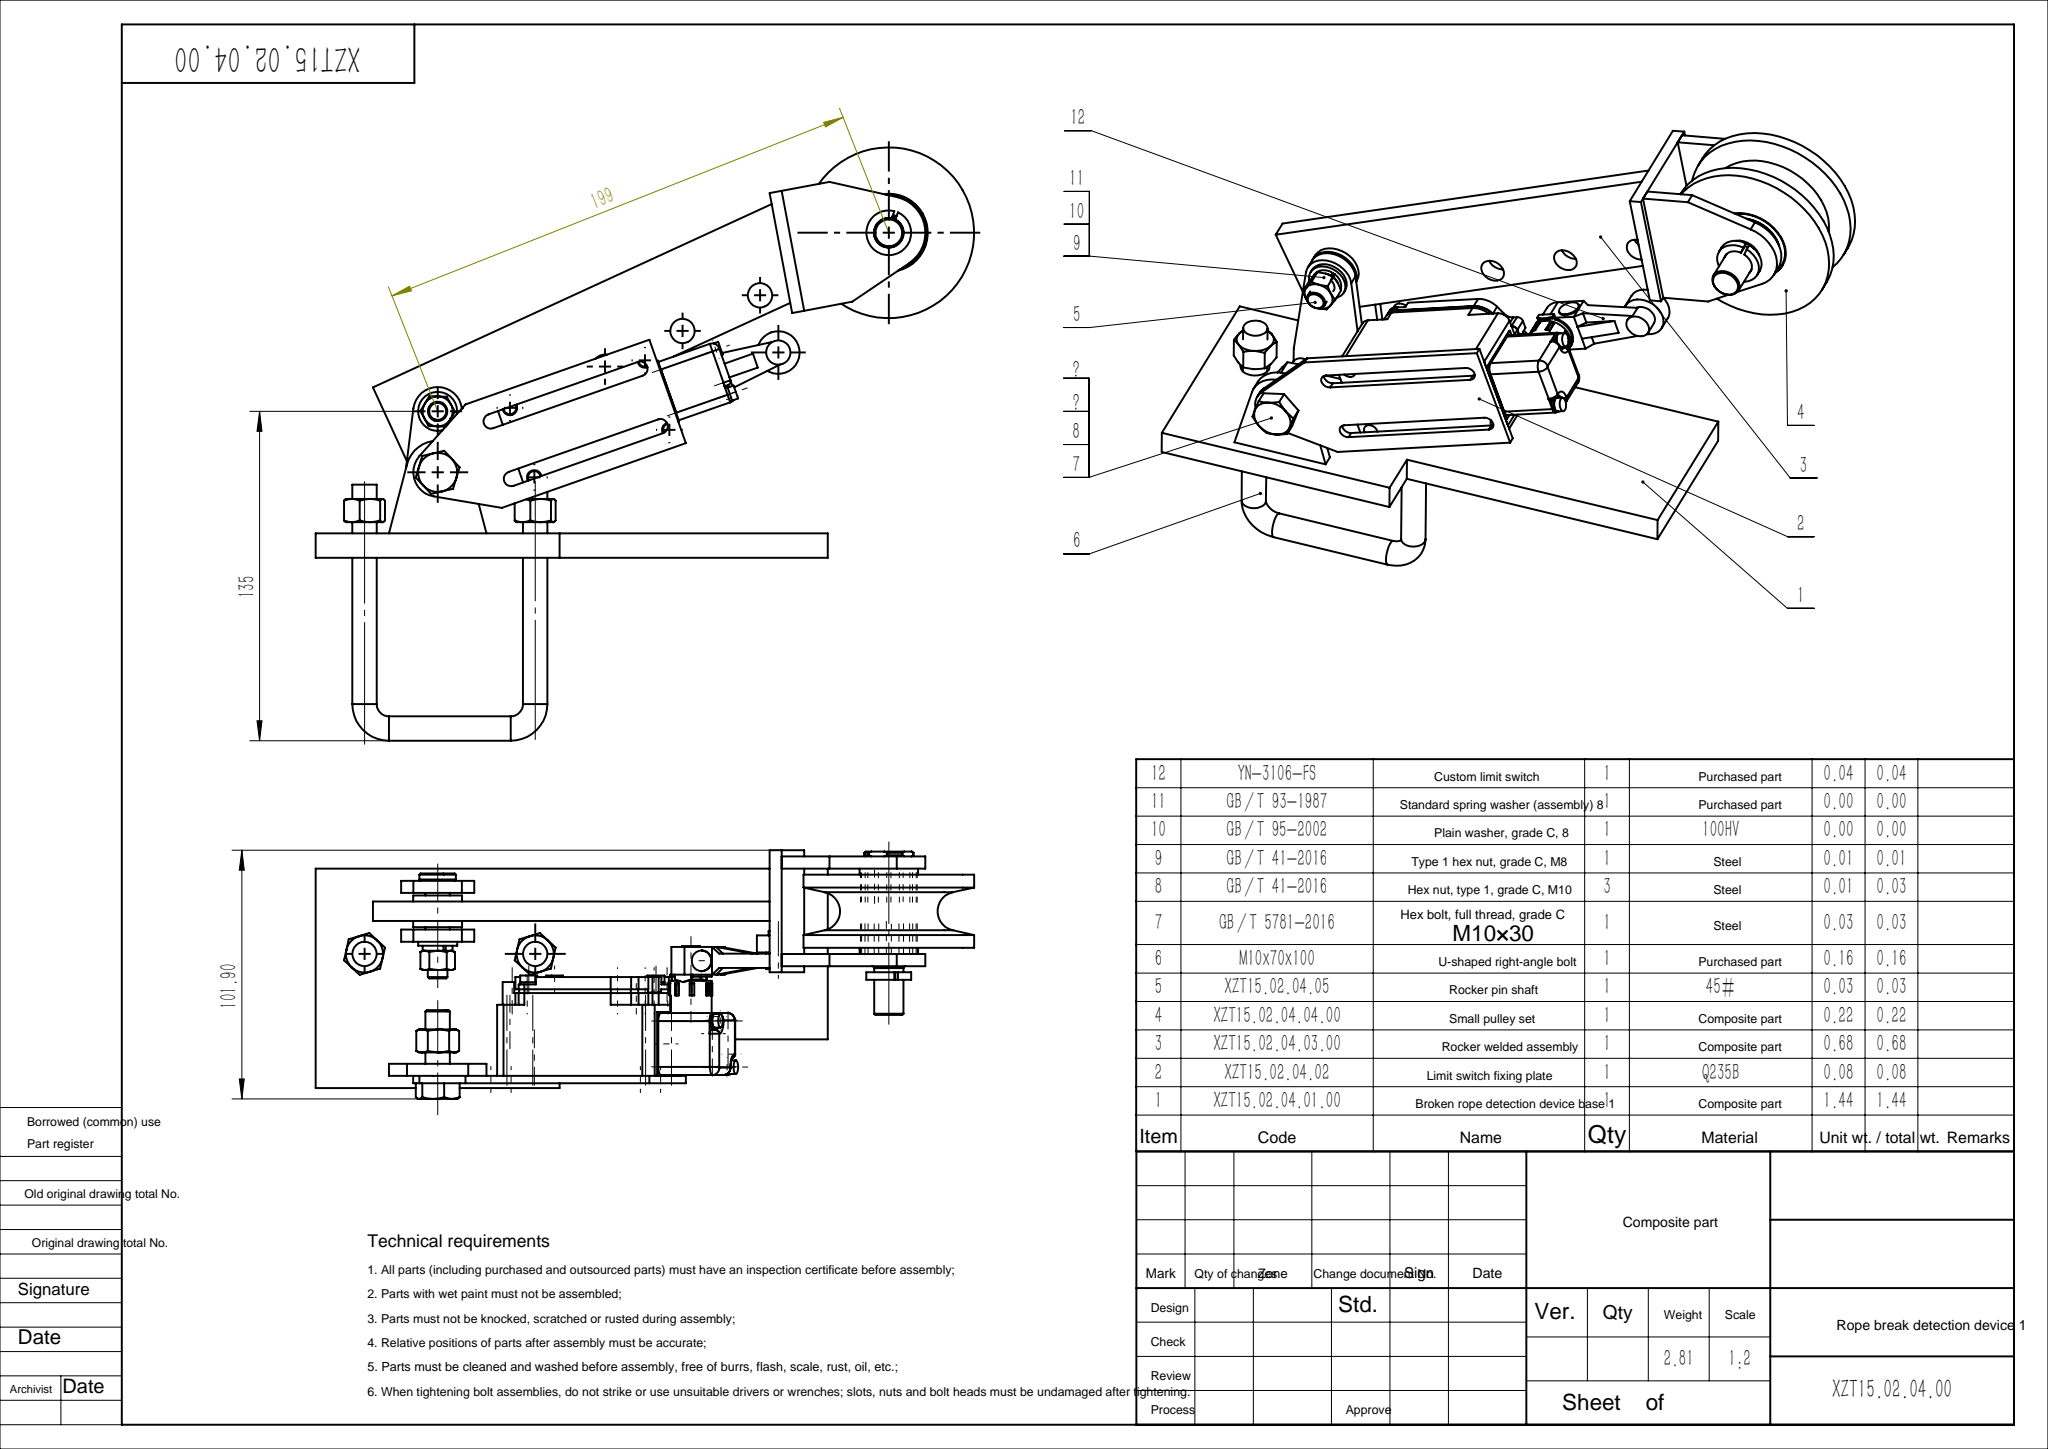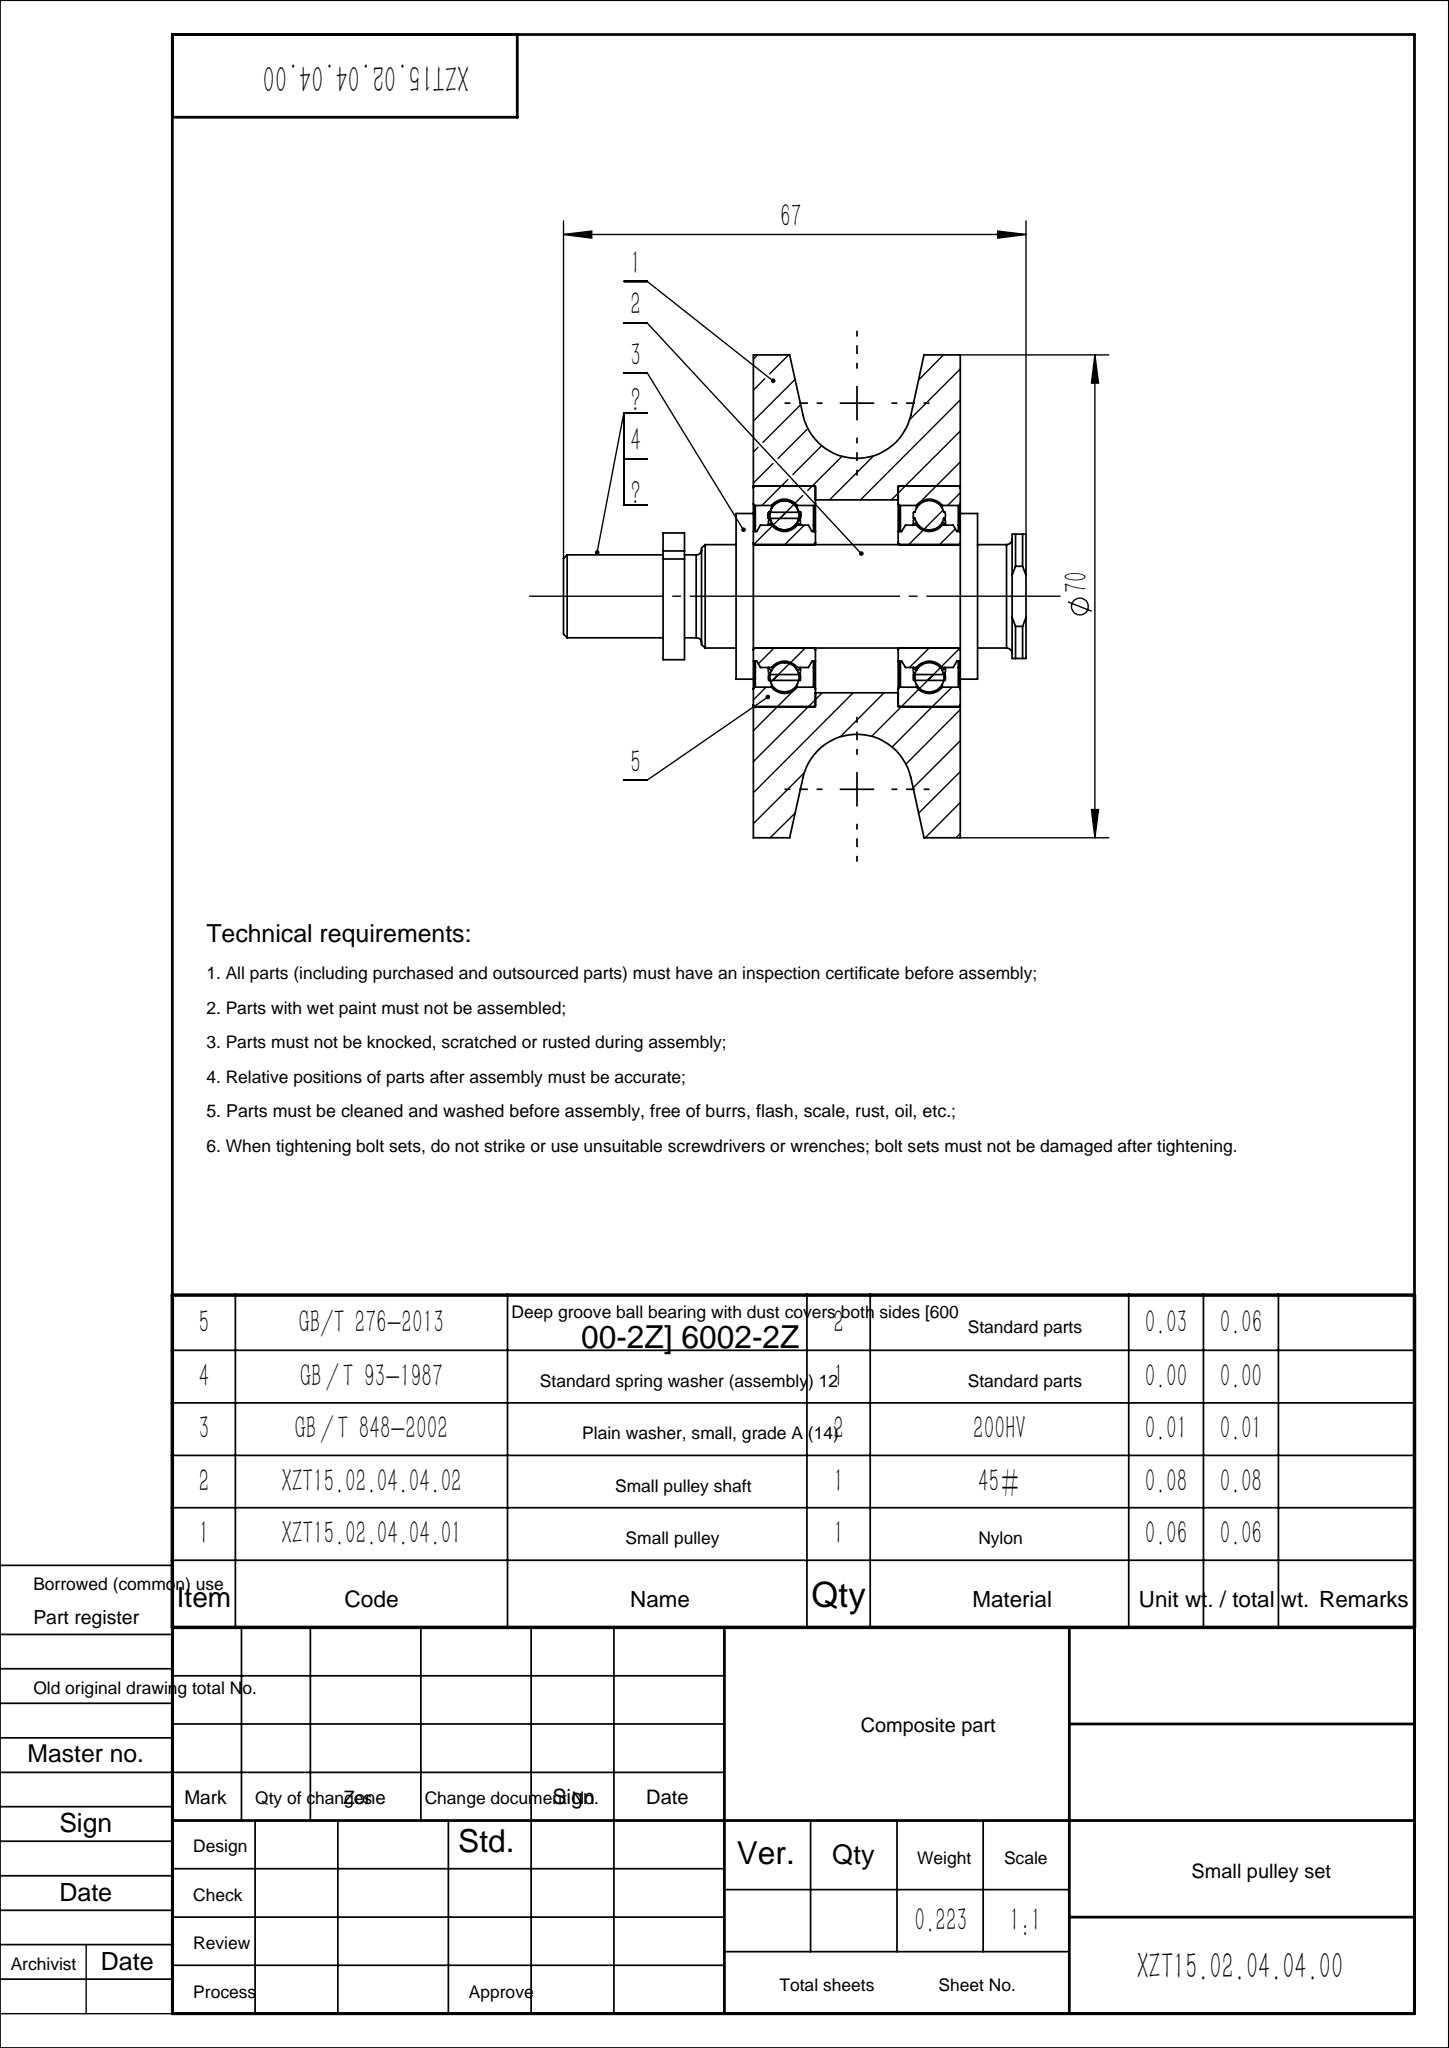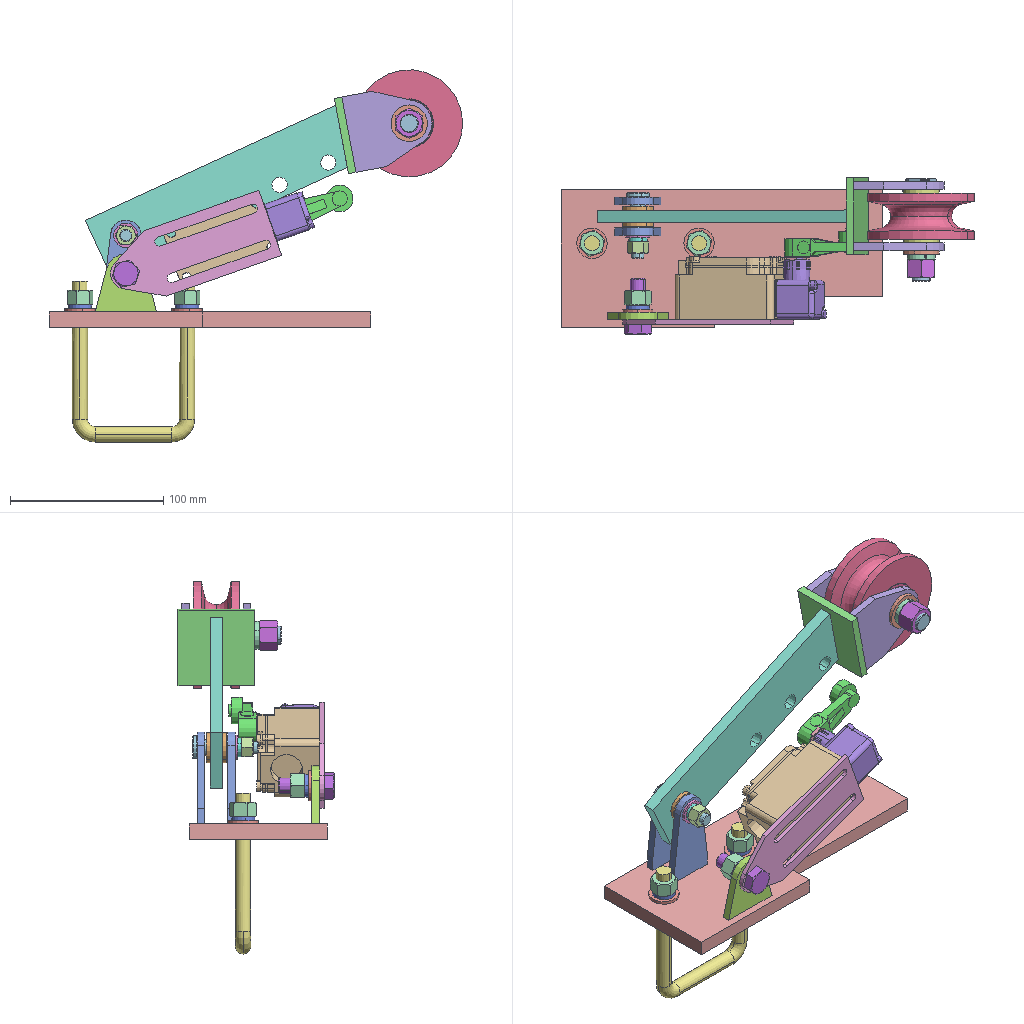Assembly | SolidWorks | 32 different items | 42 placed | box 270 x 102 x 243 mm
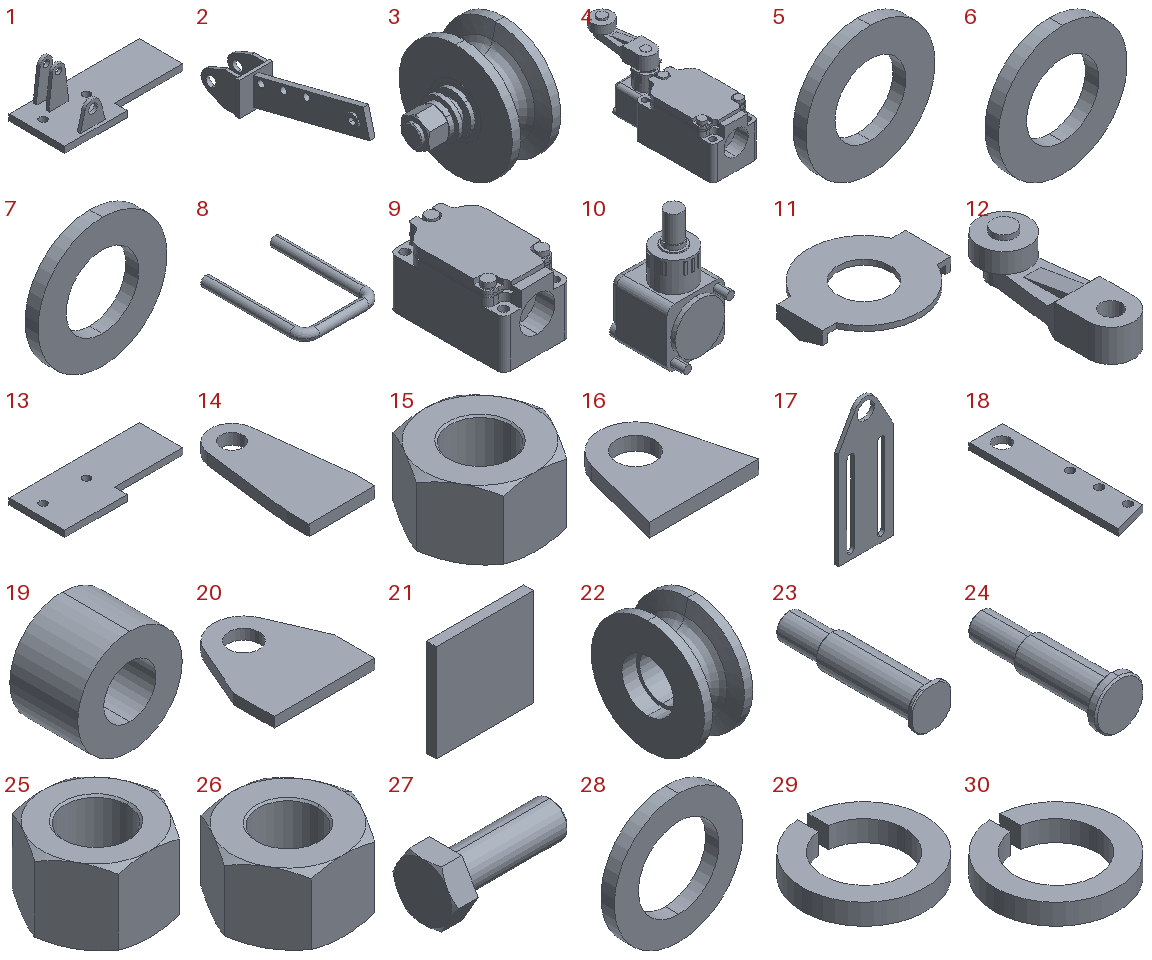Parts list (item | name | quantity | parent item | size | volume | features):
1 | (subassembly) | x1 | - | 210 x 90 x 70 mm | 183297 mm3 | -
2 | (subassembly) | x1 | - | 50 x 234.626 x 87 mm | 87256 mm3 | features MirrorCompFeat 1, ReferencePattern 1
3 | (subassembly) | x1 | - | 67 x 70 x 70 mm | 76949 mm3 | -
4 | (subassembly) | x1 | - | 40 x 125.15 x 59.4 mm | 125288 mm3 | -
5 | - | x3 | - | 20 x 2 x 20 mm | 438.252 mm3 | features Revolution 1
6 | - | x1 | in 3 | 24 x 2.5 x 24 mm | 773.126 mm3 | features Revolution 1
7 | - | x1 | - | 16 x 1.6 x 16 mm | 219.911 mm3 | features Revolution 1
8 | - | x1 | - | 80 x 105 x 10 mm | 20532 mm3 | features Sweep 1
9 | - | x1 | in 4 | 40 x 68.7 x 41.2 mm | 97429 mm3 | features BaseBody 1
10 | - | x1 | in 4 | 25.4 x 31.9 x 52.8 mm | 20430 mm3 | features BaseBody 1
11 | - | x1 | in 4 | 19.8 x 17 x 3 mm | 178.855 mm3 | features BaseBody 1
12 | - | x1 | in 4 | 17.5 x 54.75 x 17.9 mm | 7250 mm3 | features BaseBody 1
13 | - | x1 | in 1 | 210 x 90 x 10 mm | 164738 mm3 | features Extrusion 1, HoleWzd 1
14 | - | x2 | in 1 | 30 x 60 x 5 mm | 6908 mm3 | features Extrusion 1, ICE 1
15 | - | x3 | - | 17.6 x 15.242 x 9.5 mm | 1379 mm3 | features Cut 2, Chamfer 1, Extrusion 1
16 | - | x1 | in 1 | 40 x 38 x 5 mm | 4743 mm3 | features Extrusion 1
17 | - | x1 | - | 45 x 3 x 110 mm | 10350 mm3 | features Extrusion 1
18 | - | x1 | in 2 | 40 x 180 x 8 mm | 51602 mm3 | features Extrusion 1
19 | - | x1 | in 2 | 20 x 13 x 20 mm | 3063 mm3 | features Extrusion 1
20 | - | x2 | in 2 | 50 x 55 x 5 mm | 10045 mm3 | features Extrusion 1, ICE 1
21 | - | x1 | in 2 | 50 x 5 x 50 mm | 12500 mm3 | features Extrusion 1
22 | - | x1 | in 3 | 30 x 70 x 70 mm | 53072 mm3 | features Revolution 1
23 | - | x1 | in 3 | 18 x 67 x 18 mm | 10790 mm3 | features Chamfer 1, Fillet 1, ICE 1, Revolution 1
24 | - | x1 | - | 15 x 43 x 15 mm | 3230 mm3 | features Chamfer 2, Revolution 1
25 | - | x1 | in 3 | 19.9 x 17.234 x 12.2 mm | 2145 mm3 | features Cut 2, Chamfer 1, Extrusion 1
26 | - | x1 | - | 14.2 x 12.298 x 7.9 mm | 755.642 mm3 | features Cut 2, Chamfer 1, Extrusion 1
27 | - | x1 | - | 36.4 x 18.475 x 16 mm | 3775 mm3 | features Chamfer 2, RevCut 2, Revolution 2, Extrusion 1, ICE 1
28 | - | x2 | in 3 | 24 x 2.5 x 24 mm | 689.187 mm3 | features Revolution 1
29 | - | x3 | - | 15.372 x 15.344 x 2.6 mm | 261.313 mm3 | features Extrusion 1
30 | - | x1 | in 3 | 18.367 x 18.334 x 3.1 mm | 444.091 mm3 | features Extrusion 1
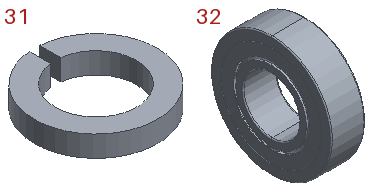31 | - | x1 | - | 12.277 x 12.254 x 2.1 mm | 135.755 mm3 | features Extrusion 1
32 | - | x2 | in 3 | 9 x 32 x 32 mm | 4173 mm3 | features Revolution 5, CirPattern 2, RefAxis 1, RevCut 1
Mates (type | each side: item.copy, entity, surface, feature):
In the top assembly
Coordinate | 1.1 select_type:25 | assembly select_type:11
Concentric | 14.1 face cylinder Boss-Extrude1 | 19.1 face cylinder Boss-Extrude1
Concentric | 20.1 face cylinder Boss-Extrude1 | 22.1 face cylinder Revolve1
Coincident | 20.1 face plane Boss-Extrude1 | 28.1 face plane Boss-Revolve
Concentric | 27.1 face cylinder Revolve1 | 15.1 face cylinder Boss-Extrude
Concentric | 27.1 face cylinder Revolve1 | 29.1 face cylinder Extrude1
Concentric | 27.1 face cylinder Revolve1 | 5.1 face cylinder Boss-Revolve
Concentric | 27.1 face cylinder Revolve1 | 17.1 face cylinder Boss-Extrude1
Concentric | 16.1 face cylinder Boss-Extrude1 | 27.1 face cylinder Revolve1
Coincident | 29.1 face plane Extrude1 | 15.1 face plane Boss-Extrude
Concentric | 24.1 face cylinder Revolve1 | 31.1 face cylinder Extrude1
Concentric | 24.1 face cylinder Revolve1 | 26.1 face cylinder Boss-Extrude
Concentric | 24.1 face cylinder Revolve1 | 7.1 face cylinder Boss-Revolve
Concentric | 24.1 face cylinder Revolve1 | 14.2 face cylinder Boss-Extrude1
Coincident | 31.1 face plane Extrude1 | 7.1 face plane Boss-Revolve
Coincident | 31.1 face plane Extrude1 | 26.1 face plane Boss-Extrude
Coincident | 14.2 face plane Boss-Extrude1 | 7.1 face plane Boss-Revolve
Coincident | 14.1 face plane Boss-Extrude1 | 24.1 face plane Revolve1
Width | 14.1 face plane Boss-Extrude1 | 14.2 face plane Boss-Extrude1 | 18.1 face plane Boss-Extrude1 | 18.1 face plane Boss-Extrude1
Coincident | 29.2 face plane Extrude1 | 15.2 face plane Boss-Extrude
Coincident | 29.2 face plane Extrude1 | 5.2 face plane Boss-Revolve
Concentric | 29.2 face cylinder Extrude1 | 15.2 face cylinder Boss-Extrude
Concentric | 29.2 face cylinder Extrude1 | 5.2 face cylinder Boss-Revolve
Concentric | 13.1 face cylinder Ø12.0 (12) Diameter Hole1 | 8.1 face cylinder Sweep1 | 2 times
Concentric | 8.1 face cylinder Sweep1 | 15.2 face cylinder Boss-Extrude
Coincident | 13.1 face plane Boss-Extrude1 | 5.2 face plane Boss-Revolve
DistanceDim | 8.1 face plane Sweep1 | 13.1 face plane Boss-Extrude1
Coincident | 17.1 face plane Boss-Extrude1 | 9.1 face plane Imported1 | 2 times
Width | 9.1 face plane Imported1 | 9.1 face plane Imported1 | 17.1 face plane Boss-Extrude1 | 17.1 face plane Boss-Extrude1
Coincident | 17.1 face plane Boss-Extrude1 | 27.1 face plane Boss-Extrude1
Coincident | 16.1 face plane Boss-Extrude1 | 17.1 face plane Boss-Extrude1
Coincident | 16.1 face plane Boss-Extrude1 | 5.1 face plane Boss-Revolve
Coincident | 5.1 face plane Boss-Revolve | 29.1 face plane Extrude1
In subassembly 4
Concentric | 9.2 face cylinder Imported1 | 10.1 face cylinder Imported1 | 2 times
Concentric | 10.1 face cylinder Imported1 | 12.1 face cylinder Imported1
DistanceDim | 9.2 face plane Imported1 | 12.1 face plane Imported1
Concentric | 10.1 face cylinder Imported1 | 11.1 face cylinder Imported1
Coincident | 12.1 face plane Imported1 | 11.1 face plane Imported1
In subassembly 1
Coordinate | 13.2 select_type:25 | 1.2 select_type:11
Coincident | 14.3 face plane Boss-Extrude2 | 14.4 face plane Boss-Extrude2 | 2 times
Coincident | 13.2 face plane Boss-Extrude1 | 14.3 face plane Boss-Extrude2
Coincident | 13.2 face plane Boss-Extrude1 | 16.2 face plane Boss-Extrude1
DistanceDim | 14.3 face plane Boss-Extrude1 | 13.2 face plane Boss-Extrude1
DistanceDim | 14.4 face plane Boss-Extrude1 | 13.2 face plane Boss-Extrude1
DistanceDim | 16.2 face plane Boss-Extrude1 | 13.2 face plane Boss-Extrude1
DistanceDim | 14.3 face cylinder Boss-Extrude1 | 13.2 face plane Boss-Extrude1
DistanceDim | 16.2 face cylinder Boss-Extrude1 | 13.2 face plane Boss-Extrude1
In subassembly 2
Coordinate | 21.1 select_type:25 | 2.1 select_type:11
Coincident | 20.2 face plane Boss-Extrude2 | 21.1 face plane Boss-Extrude1 | 2 times
DistanceDim | 20.3 face plane Boss-Extrude1 | 20.2 face plane Boss-Extrude1
Coincident | 18.2 face plane Boss-Extrude1 | 21.1 face plane Boss-Extrude1
Concentric | 18.2 face cylinder Boss-Extrude1 | 19.2 face cylinder Boss-Extrude1
Width | 19.2 face plane Boss-Extrude1 | 19.2 face plane Boss-Extrude1 | 18.2 face plane Boss-Extrude1 | 18.2 face plane Boss-Extrude1
Width | 18.2 face plane Boss-Extrude1 | 18.2 face plane Boss-Extrude1 | 21.1 face plane Boss-Extrude1 | 21.1 face plane Boss-Extrude1
DistanceDim | 21.1 face plane Boss-Extrude1 | 18.2 edge
In subassembly 3
Coordinate | 22.2 select_type:25 | 3.1 select_type:11
Concentric | 22.2 face cylinder Revolve1 | 23.1 face cylinder Revolve1
Concentric | 22.2 face cylinder Revolve1 | 28.2 face cylinder Boss-Revolve
Concentric | 22.2 face cylinder Revolve1 | 32.1 face cylinder Revolve1
Concentric | 22.2 face cylinder Revolve1 | 32.2 face cylinder Revolve1
Concentric | 22.2 face cylinder Revolve1 | 28.3 face cylinder Boss-Revolve
Concentric | 22.2 face cylinder Revolve1 | 6.1 face cylinder Boss-Revolve
Concentric | 22.2 face cylinder Revolve1 | 30.1 face cylinder Extrude1
Concentric | 22.2 face cylinder Revolve1 | 25.1 face cylinder Boss-Extrude
Coincident | 22.2 face plane Revolve1 | 32.2 face plane Revolve1
Coincident | 22.2 face plane Revolve1 | 32.1 face plane Revolve1
Coincident | 32.1 face plane Revolve1 | 28.2 face plane Boss-Revolve
DistanceDim | 23.1 face plane Revolve1 | 28.2 face plane Boss-Revolve
Coincident | 28.3 face plane Boss-Revolve | 32.2 face plane Revolve1
Coincident | 23.1 face plane Revolve1 | 6.1 face plane Boss-Revolve
Coincident | 30.1 face plane Extrude1 | 6.1 face plane Boss-Revolve
Coincident | 25.1 face plane Boss-Extrude | 30.1 face plane Extrude1
Parallel | 23.1 face plane Cut-Extrude1 | 3.1 plane